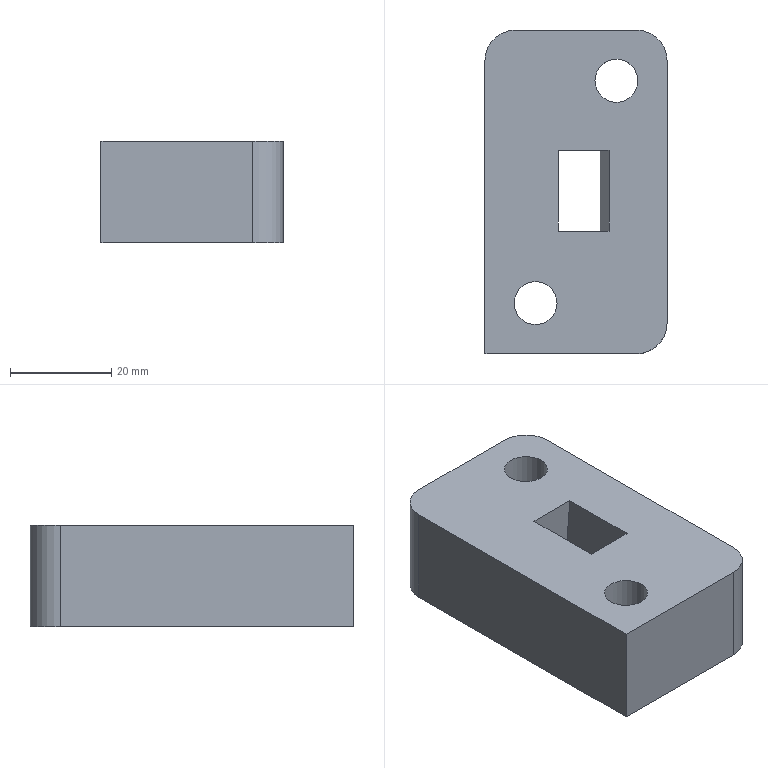Part | STEP file | solid 101 | 1 solid | 34 faces | box 36 x 64 x 20 mm | volume 38384 mm3 | plane 21 | cylinder 7 | other 6 | commonest cylinder face diameters 12 x3 8.5 x2 14 x2